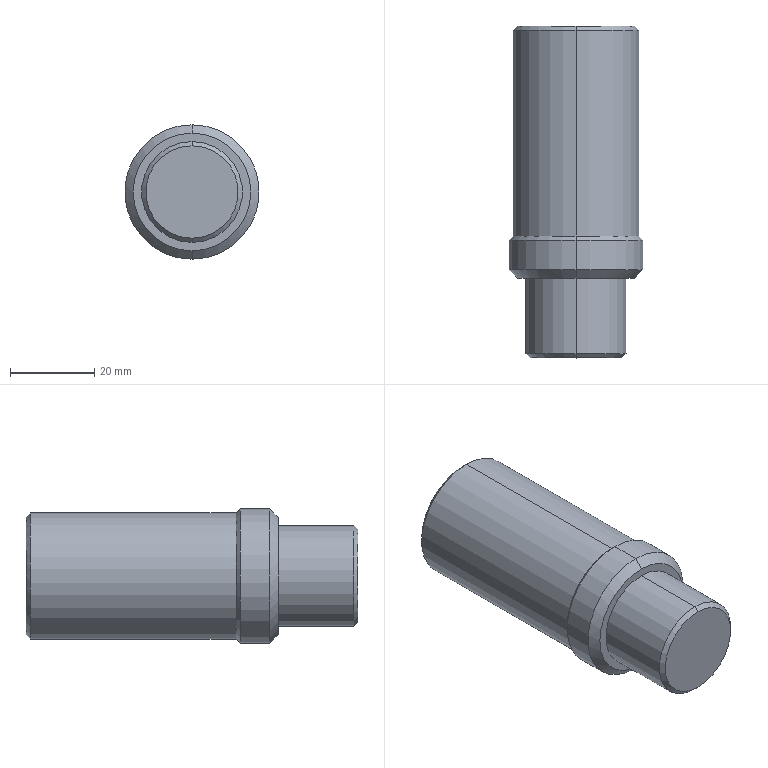Part | SolidWorks | features BaseBody 1 | 1 solid | 17 faces | box 32 x 79 x 32 mm | volume 51656 mm3 | cone 8 | cylinder 6 | plane 3 | commonest cylinder face diameters 24 x2 30 x2 32 x2
STEP:
#1=CARTESIAN_POINT('',(0.,29.,15.));
#2=VERTEX_POINT('',#1);
#3=CARTESIAN_POINT('',(0.,29.,-15.));
#4=VERTEX_POINT('',#3);
#5=CARTESIAN_POINT('',(0.,29.,0.));
#6=DIRECTION('',(0.,1.,0.));
#7=DIRECTION('',(0.,0.,1.));
#8=AXIS2_PLACEMENT_3D('',#5,#6,#7);
#9=CIRCLE('',#8,15.);
#10=EDGE_CURVE('',#2,#4,#9,.T.);
#11=ORIENTED_EDGE('',*,*,#10,.T.);
#12=CARTESIAN_POINT('',(0.,78.,-15.));
#13=VERTEX_POINT('',#12);
#14=CARTESIAN_POINT('',(0.,54.,-15.));
#15=DIRECTION('',(0.,1.,0.));
#16=VECTOR('',#15,1000.);
#17=LINE('',#14,#16);
#18=EDGE_CURVE('',#4,#13,#17,.T.);
#19=ORIENTED_EDGE('',*,*,#18,.T.);
#20=CARTESIAN_POINT('',(0.,78.,15.));
#21=VERTEX_POINT('',#20);
#22=CARTESIAN_POINT('',(0.,78.,0.));
#23=DIRECTION('',(0.,-1.,0.));
#24=DIRECTION('',(0.,0.,1.));
#25=AXIS2_PLACEMENT_3D('',#22,#23,#24);
#26=CIRCLE('',#25,15.);
#27=EDGE_CURVE('',#13,#21,#26,.T.);
#28=ORIENTED_EDGE('',*,*,#27,.T.);
#29=CARTESIAN_POINT('',(0.,54.,15.));
#30=DIRECTION('',(0.,1.,0.));
#31=VECTOR('',#30,1000.);
#32=LINE('',#29,#31);
#33=EDGE_CURVE('',#2,#21,#32,.T.);
#34=ORIENTED_EDGE('',*,*,#33,.F.);
#35=EDGE_LOOP('',(#11,#19,#28,#34));
#36=FACE_OUTER_BOUND('',#35,.T.);
#37=CARTESIAN_POINT('',(0.,54.,0.));
#38=DIRECTION('',(0.,1.,0.));
#39=DIRECTION('',(0.,0.,1.));
#40=AXIS2_PLACEMENT_3D('',#37,#38,#39);
#41=CYLINDRICAL_SURFACE('',#40,15.);
#42=ADVANCED_FACE('',(#36),#41,.T.);
#43=CARTESIAN_POINT('',(0.,79.,-14.));
#44=VERTEX_POINT('',#43);
#45=CARTESIAN_POINT('',(0.,79.,14.));
#46=VERTEX_POINT('',#45);
#47=CARTESIAN_POINT('',(0.,79.,0.));
#48=DIRECTION('',(0.,-1.,0.));
#49=DIRECTION('',(0.,0.,-1.));
#50=AXIS2_PLACEMENT_3D('',#47,#48,#49);
#51=CIRCLE('',#50,14.);
#52=EDGE_CURVE('',#44,#46,#51,.T.);
#53=ORIENTED_EDGE('',*,*,#52,.T.);
#54=CARTESIAN_POINT('',(0.,78.,15.));
#55=DIRECTION('',(0.,-0.7071,0.7071));
#56=VECTOR('',#55,1000.);
#57=LINE('',#54,#56);
#58=EDGE_CURVE('',#46,#21,#57,.T.);
#59=ORIENTED_EDGE('',*,*,#58,.T.);
#60=ORIENTED_EDGE('',*,*,#27,.F.);
#61=CARTESIAN_POINT('',(0.,78.,-15.));
#62=DIRECTION('',(0.,-0.7071,-0.7071));
#63=VECTOR('',#62,1000.);
#64=LINE('',#61,#63);
#65=EDGE_CURVE('',#44,#13,#64,.T.);
#66=ORIENTED_EDGE('',*,*,#65,.F.);
#67=EDGE_LOOP('',(#53,#59,#60,#66));
#68=FACE_OUTER_BOUND('',#67,.T.);
#69=CARTESIAN_POINT('',(0.,78.,0.));
#70=DIRECTION('',(0.,-1.,0.));
#71=DIRECTION('',(0.,0.,-1.));
#72=AXIS2_PLACEMENT_3D('',#69,#70,#71);
#73=CONICAL_SURFACE('',#72,15.,0.7854);
#74=ADVANCED_FACE('',(#68),#73,.T.);
#75=ORIENTED_EDGE('',*,*,#10,.F.);
#76=CARTESIAN_POINT('',(0.,28.,16.));
#77=VERTEX_POINT('',#76);
#78=CARTESIAN_POINT('',(0.,28.,16.));
#79=DIRECTION('',(0.,-0.7071,0.7071));
#80=VECTOR('',#79,1000.);
#81=LINE('',#78,#80);
#82=EDGE_CURVE('',#2,#77,#81,.T.);
#83=ORIENTED_EDGE('',*,*,#82,.T.);
#84=CARTESIAN_POINT('',(0.,28.,-16.));
#85=VERTEX_POINT('',#84);
#86=CARTESIAN_POINT('',(0.,28.,0.));
#87=DIRECTION('',(0.,1.,0.));
#88=DIRECTION('',(0.,0.,-1.));
#89=AXIS2_PLACEMENT_3D('',#86,#87,#88);
#90=CIRCLE('',#89,16.);
#91=EDGE_CURVE('',#77,#85,#90,.T.);
#92=ORIENTED_EDGE('',*,*,#91,.T.);
#93=CARTESIAN_POINT('',(0.,28.,-16.));
#94=DIRECTION('',(0.,-0.7071,-0.7071));
#95=VECTOR('',#94,1000.);
#96=LINE('',#93,#95);
#97=EDGE_CURVE('',#4,#85,#96,.T.);
#98=ORIENTED_EDGE('',*,*,#97,.F.);
#99=EDGE_LOOP('',(#75,#83,#92,#98));
#100=FACE_OUTER_BOUND('',#99,.T.);
#101=CARTESIAN_POINT('',(0.,28.,0.));
#102=DIRECTION('',(0.,-1.,0.));
#103=DIRECTION('',(0.,0.,-1.));
#104=AXIS2_PLACEMENT_3D('',#101,#102,#103);
#105=CONICAL_SURFACE('',#104,16.,0.7854);
#106=ADVANCED_FACE('',(#100),#105,.T.);
#107=CARTESIAN_POINT('',(0.,21.,16.));
#108=VERTEX_POINT('',#107);
#109=CARTESIAN_POINT('',(0.,21.,-16.));
#110=VERTEX_POINT('',#109);
#111=CARTESIAN_POINT('',(0.,21.,0.));
#112=DIRECTION('',(0.,1.,0.));
#113=DIRECTION('',(0.,0.,1.));
#114=AXIS2_PLACEMENT_3D('',#111,#112,#113);
#115=CIRCLE('',#114,16.);
#116=EDGE_CURVE('',#108,#110,#115,.T.);
#117=ORIENTED_EDGE('',*,*,#116,.T.);
#118=CARTESIAN_POINT('',(0.,24.,-16.));
#119=DIRECTION('',(0.,1.,0.));
#120=VECTOR('',#119,1000.);
#121=LINE('',#118,#120);
#122=EDGE_CURVE('',#110,#85,#121,.T.);
#123=ORIENTED_EDGE('',*,*,#122,.T.);
#124=ORIENTED_EDGE('',*,*,#91,.F.);
#125=CARTESIAN_POINT('',(0.,24.,16.));
#126=DIRECTION('',(0.,1.,0.));
#127=VECTOR('',#126,1000.);
#128=LINE('',#125,#127);
#129=EDGE_CURVE('',#108,#77,#128,.T.);
#130=ORIENTED_EDGE('',*,*,#129,.F.);
#131=EDGE_LOOP('',(#117,#123,#124,#130));
#132=FACE_OUTER_BOUND('',#131,.T.);
#133=CARTESIAN_POINT('',(0.,24.,0.));
#134=DIRECTION('',(0.,1.,0.));
#135=DIRECTION('',(0.,0.,1.));
#136=AXIS2_PLACEMENT_3D('',#133,#134,#135);
#137=CYLINDRICAL_SURFACE('',#136,16.);
#138=ADVANCED_FACE('',(#132),#137,.T.);
#139=CARTESIAN_POINT('',(0.,19.,14.));
#140=VERTEX_POINT('',#139);
#141=CARTESIAN_POINT('',(0.,19.,-14.));
#142=VERTEX_POINT('',#141);
#143=CARTESIAN_POINT('',(0.,19.,0.));
#144=DIRECTION('',(0.,1.,0.));
#145=DIRECTION('',(0.,0.,1.));
#146=AXIS2_PLACEMENT_3D('',#143,#144,#145);
#147=CIRCLE('',#146,14.);
#148=EDGE_CURVE('',#140,#142,#147,.T.);
#149=ORIENTED_EDGE('',*,*,#148,.T.);
#150=CARTESIAN_POINT('',(0.,21.,-16.));
#151=DIRECTION('',(0.,0.7071,-0.7071));
#152=VECTOR('',#151,1000.);
#153=LINE('',#150,#152);
#154=EDGE_CURVE('',#142,#110,#153,.T.);
#155=ORIENTED_EDGE('',*,*,#154,.T.);
#156=ORIENTED_EDGE('',*,*,#116,.F.);
#157=CARTESIAN_POINT('',(0.,21.,16.));
#158=DIRECTION('',(0.,0.7071,0.7071));
#159=VECTOR('',#158,1000.);
#160=LINE('',#157,#159);
#161=EDGE_CURVE('',#140,#108,#160,.T.);
#162=ORIENTED_EDGE('',*,*,#161,.F.);
#163=EDGE_LOOP('',(#149,#155,#156,#162));
#164=FACE_OUTER_BOUND('',#163,.T.);
#165=CARTESIAN_POINT('',(0.,21.,0.));
#166=DIRECTION('',(0.,1.,0.));
#167=DIRECTION('',(0.,0.,1.));
#168=AXIS2_PLACEMENT_3D('',#165,#166,#167);
#169=CONICAL_SURFACE('',#168,16.,0.7854);
#170=ADVANCED_FACE('',(#164),#169,.T.);
#171=CARTESIAN_POINT('',(0.,1.,12.));
#172=VERTEX_POINT('',#171);
#173=CARTESIAN_POINT('',(0.,1.,-12.));
#174=VERTEX_POINT('',#173);
#175=CARTESIAN_POINT('',(0.,1.,0.));
#176=DIRECTION('',(0.,1.,0.));
#177=DIRECTION('',(0.,0.,1.));
#178=AXIS2_PLACEMENT_3D('',#175,#176,#177);
#179=CIRCLE('',#178,12.);
#180=EDGE_CURVE('',#172,#174,#179,.T.);
#181=ORIENTED_EDGE('',*,*,#180,.T.);
#182=CARTESIAN_POINT('',(0.,19.,-12.));
#183=VERTEX_POINT('',#182);
#184=CARTESIAN_POINT('',(0.,9.5,-12.));
#185=DIRECTION('',(0.,1.,0.));
#186=VECTOR('',#185,1000.);
#187=LINE('',#184,#186);
#188=EDGE_CURVE('',#174,#183,#187,.T.);
#189=ORIENTED_EDGE('',*,*,#188,.T.);
#190=CARTESIAN_POINT('',(0.,19.,12.));
#191=VERTEX_POINT('',#190);
#192=CARTESIAN_POINT('',(0.,19.,0.));
#193=DIRECTION('',(0.,1.,0.));
#194=DIRECTION('',(0.,0.,1.));
#195=AXIS2_PLACEMENT_3D('',#192,#193,#194);
#196=CIRCLE('',#195,12.);
#197=EDGE_CURVE('',#191,#183,#196,.T.);
#198=ORIENTED_EDGE('',*,*,#197,.F.);
#199=CARTESIAN_POINT('',(0.,9.5,12.));
#200=DIRECTION('',(0.,1.,0.));
#201=VECTOR('',#200,1000.);
#202=LINE('',#199,#201);
#203=EDGE_CURVE('',#172,#191,#202,.T.);
#204=ORIENTED_EDGE('',*,*,#203,.F.);
#205=EDGE_LOOP('',(#181,#189,#198,#204));
#206=FACE_OUTER_BOUND('',#205,.T.);
#207=CARTESIAN_POINT('',(0.,9.5,0.));
#208=DIRECTION('',(0.,1.,0.));
#209=DIRECTION('',(0.,0.,1.));
#210=AXIS2_PLACEMENT_3D('',#207,#208,#209);
#211=CYLINDRICAL_SURFACE('',#210,12.);
#212=ADVANCED_FACE('',(#206),#211,.T.);
#213=CARTESIAN_POINT('',(0.,0.,11.));
#214=VERTEX_POINT('',#213);
#215=CARTESIAN_POINT('',(0.,0.,-11.));
#216=VERTEX_POINT('',#215);
#217=CARTESIAN_POINT('',(0.,0.,0.));
#218=DIRECTION('',(0.,1.,0.));
#219=DIRECTION('',(0.,0.,1.));
#220=AXIS2_PLACEMENT_3D('',#217,#218,#219);
#221=CIRCLE('',#220,11.);
#222=EDGE_CURVE('',#214,#216,#221,.T.);
#223=ORIENTED_EDGE('',*,*,#222,.T.);
#224=CARTESIAN_POINT('',(0.,1.,-12.));
#225=DIRECTION('',(0.,0.7071,-0.7071));
#226=VECTOR('',#225,1000.);
#227=LINE('',#224,#226);
#228=EDGE_CURVE('',#216,#174,#227,.T.);
#229=ORIENTED_EDGE('',*,*,#228,.T.);
#230=ORIENTED_EDGE('',*,*,#180,.F.);
#231=CARTESIAN_POINT('',(0.,1.,12.));
#232=DIRECTION('',(0.,0.7071,0.7071));
#233=VECTOR('',#232,1000.);
#234=LINE('',#231,#233);
#235=EDGE_CURVE('',#214,#172,#234,.T.);
#236=ORIENTED_EDGE('',*,*,#235,.F.);
#237=EDGE_LOOP('',(#223,#229,#230,#236));
#238=FACE_OUTER_BOUND('',#237,.T.);
#239=CARTESIAN_POINT('',(0.,1.,0.));
#240=DIRECTION('',(0.,1.,0.));
#241=DIRECTION('',(0.,0.,1.));
#242=AXIS2_PLACEMENT_3D('',#239,#240,#241);
#243=CONICAL_SURFACE('',#242,12.,0.7854);
#244=ADVANCED_FACE('',(#238),#243,.T.);
#245=ORIENTED_EDGE('',*,*,#18,.F.);
#246=CARTESIAN_POINT('',(0.,29.,0.));
#247=DIRECTION('',(0.,1.,0.));
#248=DIRECTION('',(0.,0.,1.));
#249=AXIS2_PLACEMENT_3D('',#246,#247,#248);
#250=CIRCLE('',#249,15.);
#251=EDGE_CURVE('',#4,#2,#250,.T.);
#252=ORIENTED_EDGE('',*,*,#251,.T.);
#253=ORIENTED_EDGE('',*,*,#33,.T.);
#254=CARTESIAN_POINT('',(0.,78.,0.));
#255=DIRECTION('',(0.,-1.,0.));
#256=DIRECTION('',(0.,0.,1.));
#257=AXIS2_PLACEMENT_3D('',#254,#255,#256);
#258=CIRCLE('',#257,15.);
#259=EDGE_CURVE('',#21,#13,#258,.T.);
#260=ORIENTED_EDGE('',*,*,#259,.T.);
#261=EDGE_LOOP('',(#245,#252,#253,#260));
#262=FACE_OUTER_BOUND('',#261,.T.);
#263=CARTESIAN_POINT('',(0.,54.,0.));
#264=DIRECTION('',(0.,1.,0.));
#265=DIRECTION('',(0.,0.,1.));
#266=AXIS2_PLACEMENT_3D('',#263,#264,#265);
#267=CYLINDRICAL_SURFACE('',#266,15.);
#268=ADVANCED_FACE('',(#262),#267,.T.);
#269=ORIENTED_EDGE('',*,*,#58,.F.);
#270=CARTESIAN_POINT('',(0.,79.,0.));
#271=DIRECTION('',(0.,-1.,0.));
#272=DIRECTION('',(0.,0.,-1.));
#273=AXIS2_PLACEMENT_3D('',#270,#271,#272);
#274=CIRCLE('',#273,14.);
#275=EDGE_CURVE('',#46,#44,#274,.T.);
#276=ORIENTED_EDGE('',*,*,#275,.T.);
#277=ORIENTED_EDGE('',*,*,#65,.T.);
#278=ORIENTED_EDGE('',*,*,#259,.F.);
#279=EDGE_LOOP('',(#269,#276,#277,#278));
#280=FACE_OUTER_BOUND('',#279,.T.);
#281=CARTESIAN_POINT('',(0.,78.,0.));
#282=DIRECTION('',(0.,-1.,0.));
#283=DIRECTION('',(0.,0.,-1.));
#284=AXIS2_PLACEMENT_3D('',#281,#282,#283);
#285=CONICAL_SURFACE('',#284,15.,0.7854);
#286=ADVANCED_FACE('',(#280),#285,.T.);
#287=ORIENTED_EDGE('',*,*,#82,.F.);
#288=ORIENTED_EDGE('',*,*,#251,.F.);
#289=ORIENTED_EDGE('',*,*,#97,.T.);
#290=CARTESIAN_POINT('',(0.,28.,0.));
#291=DIRECTION('',(0.,1.,0.));
#292=DIRECTION('',(0.,0.,-1.));
#293=AXIS2_PLACEMENT_3D('',#290,#291,#292);
#294=CIRCLE('',#293,16.);
#295=EDGE_CURVE('',#85,#77,#294,.T.);
#296=ORIENTED_EDGE('',*,*,#295,.T.);
#297=EDGE_LOOP('',(#287,#288,#289,#296));
#298=FACE_OUTER_BOUND('',#297,.T.);
#299=CARTESIAN_POINT('',(0.,28.,0.));
#300=DIRECTION('',(0.,-1.,0.));
#301=DIRECTION('',(0.,0.,-1.));
#302=AXIS2_PLACEMENT_3D('',#299,#300,#301);
#303=CONICAL_SURFACE('',#302,16.,0.7854);
#304=ADVANCED_FACE('',(#298),#303,.T.);
#305=ORIENTED_EDGE('',*,*,#52,.F.);
#306=ORIENTED_EDGE('',*,*,#275,.F.);
#307=EDGE_LOOP('',(#305,#306));
#308=FACE_OUTER_BOUND('',#307,.T.);
#309=CARTESIAN_POINT('',(0.,79.,7.5));
#310=DIRECTION('',(0.,1.,0.));
#311=DIRECTION('',(0.,0.,1.));
#312=AXIS2_PLACEMENT_3D('',#309,#310,#311);
#313=PLANE('',#312);
#314=ADVANCED_FACE('',(#308),#313,.T.);
#315=ORIENTED_EDGE('',*,*,#122,.F.);
#316=CARTESIAN_POINT('',(0.,21.,0.));
#317=DIRECTION('',(0.,1.,0.));
#318=DIRECTION('',(0.,0.,1.));
#319=AXIS2_PLACEMENT_3D('',#316,#317,#318);
#320=CIRCLE('',#319,16.);
#321=EDGE_CURVE('',#110,#108,#320,.T.);
#322=ORIENTED_EDGE('',*,*,#321,.T.);
#323=ORIENTED_EDGE('',*,*,#129,.T.);
#324=ORIENTED_EDGE('',*,*,#295,.F.);
#325=EDGE_LOOP('',(#315,#322,#323,#324));
#326=FACE_OUTER_BOUND('',#325,.T.);
#327=CARTESIAN_POINT('',(0.,24.,0.));
#328=DIRECTION('',(0.,1.,0.));
#329=DIRECTION('',(0.,0.,1.));
#330=AXIS2_PLACEMENT_3D('',#327,#328,#329);
#331=CYLINDRICAL_SURFACE('',#330,16.);
#332=ADVANCED_FACE('',(#326),#331,.T.);
#333=ORIENTED_EDGE('',*,*,#154,.F.);
#334=CARTESIAN_POINT('',(0.,19.,0.));
#335=DIRECTION('',(0.,1.,0.));
#336=DIRECTION('',(0.,0.,1.));
#337=AXIS2_PLACEMENT_3D('',#334,#335,#336);
#338=CIRCLE('',#337,14.);
#339=EDGE_CURVE('',#142,#140,#338,.T.);
#340=ORIENTED_EDGE('',*,*,#339,.T.);
#341=ORIENTED_EDGE('',*,*,#161,.T.);
#342=ORIENTED_EDGE('',*,*,#321,.F.);
#343=EDGE_LOOP('',(#333,#340,#341,#342));
#344=FACE_OUTER_BOUND('',#343,.T.);
#345=CARTESIAN_POINT('',(0.,21.,0.));
#346=DIRECTION('',(0.,1.,0.));
#347=DIRECTION('',(0.,0.,1.));
#348=AXIS2_PLACEMENT_3D('',#345,#346,#347);
#349=CONICAL_SURFACE('',#348,16.,0.7854);
#350=ADVANCED_FACE('',(#344),#349,.T.);
#351=ORIENTED_EDGE('',*,*,#197,.T.);
#352=CARTESIAN_POINT('',(0.,19.,0.));
#353=DIRECTION('',(0.,1.,0.));
#354=DIRECTION('',(0.,0.,1.));
#355=AXIS2_PLACEMENT_3D('',#352,#353,#354);
#356=CIRCLE('',#355,12.);
#357=EDGE_CURVE('',#183,#191,#356,.T.);
#358=ORIENTED_EDGE('',*,*,#357,.T.);
#359=EDGE_LOOP('',(#351,#358));
#360=FACE_BOUND('',#359,.T.);
#361=ORIENTED_EDGE('',*,*,#148,.F.);
#362=ORIENTED_EDGE('',*,*,#339,.F.);
#363=EDGE_LOOP('',(#361,#362));
#364=FACE_OUTER_BOUND('',#363,.T.);
#365=CARTESIAN_POINT('',(0.,19.,14.));
#366=DIRECTION('',(0.,-1.,0.));
#367=DIRECTION('',(0.,0.,-1.));
#368=AXIS2_PLACEMENT_3D('',#365,#366,#367);
#369=PLANE('',#368);
#370=ADVANCED_FACE('',(#360,#364),#369,.T.);
#371=ORIENTED_EDGE('',*,*,#188,.F.);
#372=CARTESIAN_POINT('',(0.,1.,0.));
#373=DIRECTION('',(0.,1.,0.));
#374=DIRECTION('',(0.,0.,1.));
#375=AXIS2_PLACEMENT_3D('',#372,#373,#374);
#376=CIRCLE('',#375,12.);
#377=EDGE_CURVE('',#174,#172,#376,.T.);
#378=ORIENTED_EDGE('',*,*,#377,.T.);
#379=ORIENTED_EDGE('',*,*,#203,.T.);
#380=ORIENTED_EDGE('',*,*,#357,.F.);
#381=EDGE_LOOP('',(#371,#378,#379,#380));
#382=FACE_OUTER_BOUND('',#381,.T.);
#383=CARTESIAN_POINT('',(0.,9.5,0.));
#384=DIRECTION('',(0.,1.,0.));
#385=DIRECTION('',(0.,0.,1.));
#386=AXIS2_PLACEMENT_3D('',#383,#384,#385);
#387=CYLINDRICAL_SURFACE('',#386,12.);
#388=ADVANCED_FACE('',(#382),#387,.T.);
#389=ORIENTED_EDGE('',*,*,#228,.F.);
#390=CARTESIAN_POINT('',(0.,0.,0.));
#391=DIRECTION('',(0.,1.,0.));
#392=DIRECTION('',(0.,0.,1.));
#393=AXIS2_PLACEMENT_3D('',#390,#391,#392);
#394=CIRCLE('',#393,11.);
#395=EDGE_CURVE('',#216,#214,#394,.T.);
#396=ORIENTED_EDGE('',*,*,#395,.T.);
#397=ORIENTED_EDGE('',*,*,#235,.T.);
#398=ORIENTED_EDGE('',*,*,#377,.F.);
#399=EDGE_LOOP('',(#389,#396,#397,#398));
#400=FACE_OUTER_BOUND('',#399,.T.);
#401=CARTESIAN_POINT('',(0.,1.,0.));
#402=DIRECTION('',(0.,1.,0.));
#403=DIRECTION('',(0.,0.,1.));
#404=AXIS2_PLACEMENT_3D('',#401,#402,#403);
#405=CONICAL_SURFACE('',#404,12.,0.7854);
#406=ADVANCED_FACE('',(#400),#405,.T.);
#407=ORIENTED_EDGE('',*,*,#222,.F.);
#408=ORIENTED_EDGE('',*,*,#395,.F.);
#409=EDGE_LOOP('',(#407,#408));
#410=FACE_OUTER_BOUND('',#409,.T.);
#411=CARTESIAN_POINT('',(0.,0.,6.));
#412=DIRECTION('',(0.,-1.,0.));
#413=DIRECTION('',(0.,0.,-1.));
#414=AXIS2_PLACEMENT_3D('',#411,#412,#413);
#415=PLANE('',#414);
#416=ADVANCED_FACE('',(#410),#415,.T.);
#417=CLOSED_SHELL('',(#42,#74,#106,#138,#170,#212,#244,#268,#286,#304,#314,#332,#350,#370,#388,#406,#416));
#418=MANIFOLD_SOLID_BREP('',#417);
#419=CARTESIAN_POINT('',(0.,0.,0.));
#420=DIRECTION('',(0.,0.,1.));
#421=DIRECTION('',(1.,0.,0.));
#422=AXIS2_PLACEMENT_3D('',#419,#420,#421);
#423=(LENGTH_UNIT()NAMED_UNIT(*)SI_UNIT(.MILLI.,.METRE.));
#424=UNCERTAINTY_MEASURE_WITH_UNIT(LENGTH_MEASURE(0.00001),#423,'','');
#425=(NAMED_UNIT(*)PLANE_ANGLE_UNIT()SI_UNIT($,.RADIAN.));
#426=(NAMED_UNIT(*)SI_UNIT($,.STERADIAN.)SOLID_ANGLE_UNIT());
#427=(GEOMETRIC_REPRESENTATION_CONTEXT(3)GLOBAL_UNCERTAINTY_ASSIGNED_CONTEXT((#424))GLOBAL_UNIT_ASSIGNED_CONTEXT((#423,#425,#426))REPRESENTATION_CONTEXT('',''));
#428=ADVANCED_BREP_SHAPE_REPRESENTATION('',(#418,#422),#427);